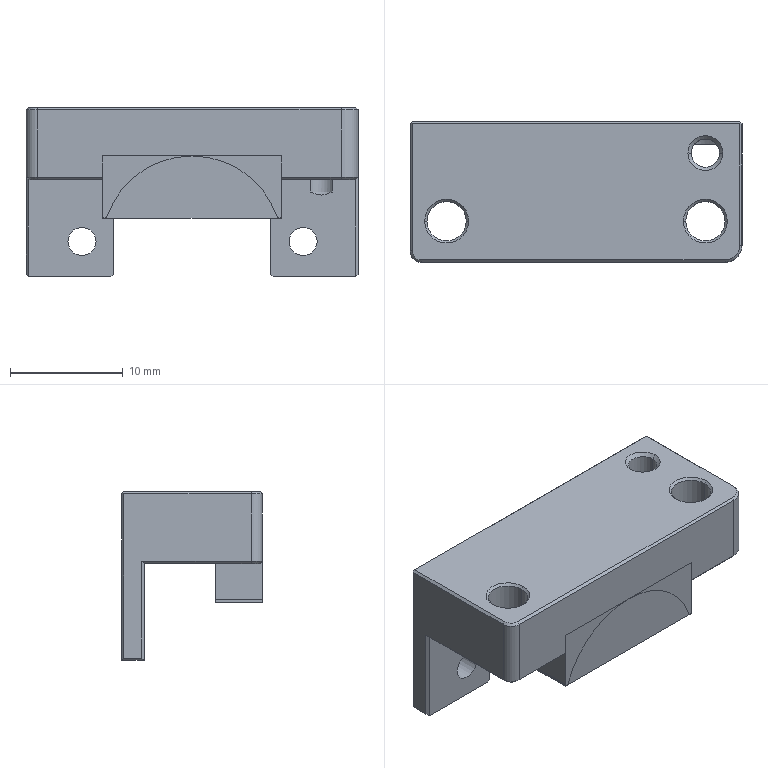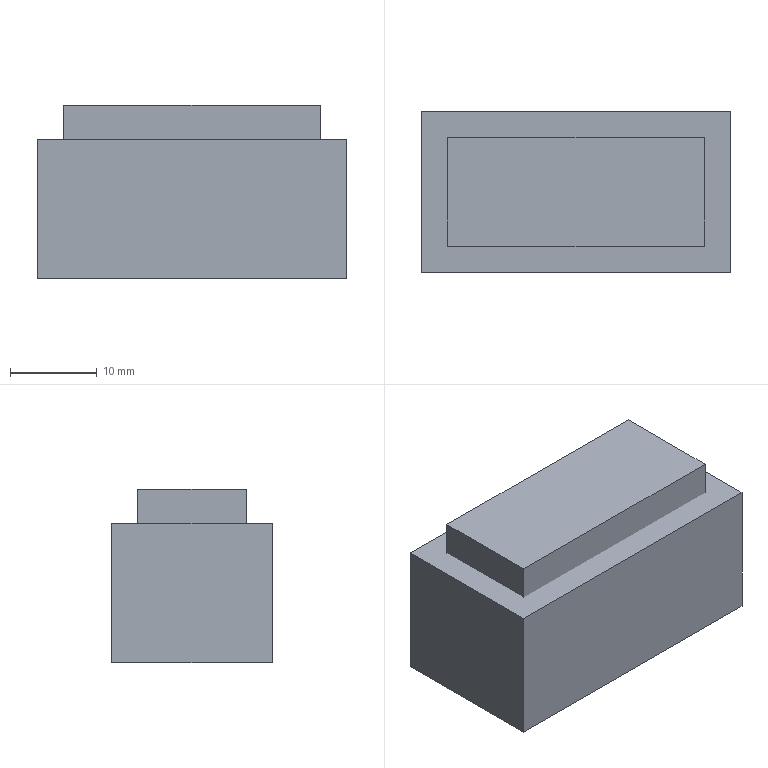CAM job | NX | 3+2 milling, drilling | part box 29.5 x 12.5 x 15 mm | stock box 35.5 x 18.5 x 20 mm
Tools:
number,name,description,diameter,corner_radius,flute_length,length,flutes
3,D63,Milling Tool-5 Parameters,63.0,0.0,50.0,75.0,2
1,D6A45,Milling Tool-5 Parameters,6.0,0.0,3.0,3.0,2
11,3.5ZT,Drilling Tool,3.5,0.0,35.0,50.0,2
16,D6JING,Milling Tool-5 Parameters,6.0,0.0,50.0,75.0,2
12,2.5ZT,Drilling Tool,2.5,0.0,35.0,50.0,2
18,D2,Milling Tool-5 Parameters,2.0,0.0,50.0,75.0,2
17,D4,Milling Tool-5 Parameters,4.0,0.0,50.0,75.0,2
Operations:
program,operation,operation_type,tool,method,geometry_group,spindle_rpm,surface_speed,feed_per_tooth,feed_cut,feed_plunge,cut_length_mm,path_length_mm,cut_time_min,machine_time_min
1,FLOOR_WALL_COPY,VolumeBased25DMillingOperation,D63,METHOD,A,6500.0,1286.0,0.0962,1250.0,100.0,104.498,158.498,0.0836,0.089
1,DRILLING_COPY_1,Operation,D6A45,METHOD,A,5000.0,94.0,0.025,250.0,0.0,12.0,137.166,0.048,0.0605
1,DRILLING_COPY_1_COPY,Operation,3.5ZT,METHOD,A,2000.0,20.0,0.0625,250.0,0.0,23.903,134.001,0.0956,0.1066
1,DRILLING_COPY_1_COPY_COPY,Operation,2.5ZT,METHOD,A,2546.0,20.0,0.0295,150.0,0.0,10.77,81.541,0.0718,0.0789
1,ADAPTIVE_MILLING_COPY,CavityMilling,D6JING,METHOD,A,9500.0,179.0,0.1579,3000.0,1000.0,855.855,941.855,0.286,0.2946
1,ZLEVEL_PROFILE_1_COPY,ZLevelMilling,D6JING,METHOD,A,9500.0,298.0,0.0526,1000.0,100.0,105.425,193.425,0.1054,0.1142
1,11_COPY_COPY,ZLevelMilling,D6A45,METHOD,A,9500.0,179.0,0.0526,1000.0,100.0,134.92,432.354,0.1349,0.1647
2,FLOOR_WALL_COPY_COPY,VolumeBased25DMillingOperation,D63,METHOD,B,6500.0,1286.0,0.0962,1250.0,100.0,522.49,1166.482,0.418,0.4824
2,FLOOR_WALL,VolumeBased25DMillingOperation,D6JING,METHOD,B,9500.0,179.0,0.1316,2500.0,1000.0,3664.41,3877.666,1.511,1.533
2,FLOOR_WALL_COPY_1,VolumeBased25DMillingOperation,D6JING,METHOD,B,9500.0,179.0,0.0526,1000.0,1000.0,185.908,357.488,0.1859,0.2032
2,FLOOR_WALL_COPY_1_COPY,VolumeBased25DMillingOperation,D6JING,METHOD,B,9500.0,179.0,0.0526,1000.0,1000.0,169.057,381.37,0.1691,0.1907
2,ZLEVEL_PROFILE_1_COPY_COPY,ZLevelMilling,D6JING,METHOD,B,9500.0,298.0,0.0526,1000.0,100.0,48.391,230.204,0.0484,0.0666
2,ZLEVEL_PROFILE_COPY_COPY_COPY_1_COPY_COPY,ZLevelMilling,D2,METHOD,B,9500.0,59.0,0.0526,1000.0,1000.0,55.446,243.643,0.0554,0.0743
2,11_COPY_COPY_1,ZLevelMilling,D6A45,METHOD,B,9500.0,179.0,0.0526,1000.0,100.0,67.65,203.364,0.0676,0.0812
2,11_COPY_COPY_1_COPY,ZLevelMilling,D6A45,METHOD,B,9500.0,179.0,0.0526,1000.0,100.0,69.469,332.015,0.0695,0.0957
2,刀补16,ZLevelMilling,D6JING,METHOD,B,9500.0,298.0,0.0526,1000.0,100.0,32.022,206.923,0.032,0.0495
3,DRILLING_COPY_1_COPY_1,Operation,D6A45,METHOD,D,5000.0,94.0,0.025,250.0,0.0,8.9,100.678,0.0356,0.0448
3,DRILLING_COPY_1_COPY_COPY_COPY,Operation,2.5ZT,METHOD,D,2000.0,20.0,0.0375,150.0,0.0,14.502,111.882,0.0967,0.1064
4,ZLEVEL_PROFILE_1_COPY_COPY_COPY,ZLevelMilling,D4,METHOD,C,9500.0,298.0,0.1053,2000.0,100.0,317.108,385.508,0.1586,0.1654
4,ZLEVEL_PROFILE_1_COPY_COPY_1,ZLevelMilling,D4,METHOD,C,9500.0,298.0,0.0526,1000.0,100.0,30.514,96.914,0.0305,0.0372
4,PLANAR_MILL,PlanarMilling,D6A45,METHOD,C,9500.0,179.0,0.0658,1250.0,100.0,94.363,153.363,0.0755,0.0814